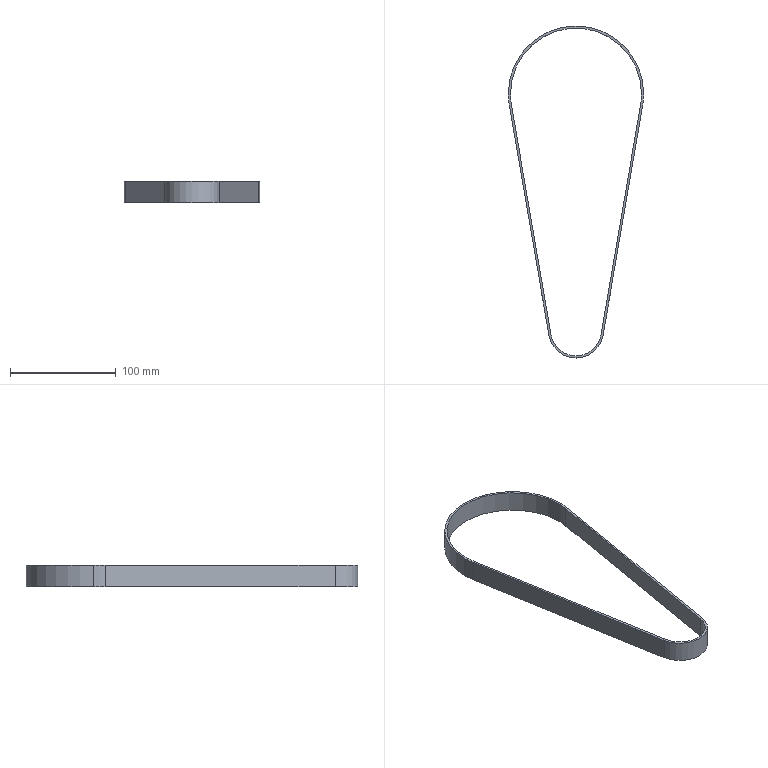Part | SolidWorks | features ExtruThin 1 | 1 solid | 14 faces | box 128 x 314 x 20 mm | volume 29237 mm3 | cylinder 8 | plane 6 | commonest cylinder face diameters 124 x3 128 x3 48 x1 52 x1
STEP:
#1=CARTESIAN_POINT('',(61.101,-10.518,20.));
#2=VERTEX_POINT('',#1);
#3=CARTESIAN_POINT('',(62.,0.,20.));
#4=VERTEX_POINT('',#3);
#5=CARTESIAN_POINT('',(0.,0.,20.));
#6=DIRECTION('',(0.,0.,1.));
#7=DIRECTION('',(1.,0.,0.));
#8=AXIS2_PLACEMENT_3D('',#5,#6,#7);
#9=CIRCLE('',#8,62.);
#10=EDGE_CURVE('',#2,#4,#9,.T.);
#11=ORIENTED_EDGE('',*,*,#10,.T.);
#12=CARTESIAN_POINT('',(62.,0.,0.));
#13=VERTEX_POINT('',#12);
#14=CARTESIAN_POINT('',(62.,0.,20.));
#15=DIRECTION('',(0.,0.,-1.));
#16=VECTOR('',#15,1000.);
#17=LINE('',#14,#16);
#18=EDGE_CURVE('',#4,#13,#17,.T.);
#19=ORIENTED_EDGE('',*,*,#18,.T.);
#20=CARTESIAN_POINT('',(61.101,-10.518,0.));
#21=VERTEX_POINT('',#20);
#22=CARTESIAN_POINT('',(0.,0.,0.));
#23=DIRECTION('',(0.,0.,1.));
#24=DIRECTION('',(1.,0.,0.));
#25=AXIS2_PLACEMENT_3D('',#22,#23,#24);
#26=CIRCLE('',#25,62.);
#27=EDGE_CURVE('',#21,#13,#26,.T.);
#28=ORIENTED_EDGE('',*,*,#27,.F.);
#29=CARTESIAN_POINT('',(61.101,-10.518,20.));
#30=DIRECTION('',(0.,0.,-1.));
#31=VECTOR('',#30,1000.);
#32=LINE('',#29,#31);
#33=EDGE_CURVE('',#2,#21,#32,.T.);
#34=ORIENTED_EDGE('',*,*,#33,.F.);
#35=EDGE_LOOP('',(#11,#19,#28,#34));
#36=FACE_OUTER_BOUND('',#35,.T.);
#37=CARTESIAN_POINT('',(0.,0.,20.));
#38=DIRECTION('',(0.,0.,-1.));
#39=DIRECTION('',(-1.,0.,0.));
#40=AXIS2_PLACEMENT_3D('',#37,#38,#39);
#41=CYLINDRICAL_SURFACE('',#40,62.);
#42=ADVANCED_FACE('',(#36),#41,.F.);
#43=ORIENTED_EDGE('',*,*,#18,.F.);
#44=CARTESIAN_POINT('',(-62.,0.,20.));
#45=VERTEX_POINT('',#44);
#46=CARTESIAN_POINT('',(0.,0.,20.));
#47=DIRECTION('',(0.,0.,1.));
#48=DIRECTION('',(1.,0.,0.));
#49=AXIS2_PLACEMENT_3D('',#46,#47,#48);
#50=CIRCLE('',#49,62.);
#51=EDGE_CURVE('',#4,#45,#50,.T.);
#52=ORIENTED_EDGE('',*,*,#51,.T.);
#53=CARTESIAN_POINT('',(-62.,0.,0.));
#54=VERTEX_POINT('',#53);
#55=CARTESIAN_POINT('',(-62.,0.,20.));
#56=DIRECTION('',(0.,0.,-1.));
#57=VECTOR('',#56,1000.);
#58=LINE('',#55,#57);
#59=EDGE_CURVE('',#45,#54,#58,.T.);
#60=ORIENTED_EDGE('',*,*,#59,.T.);
#61=CARTESIAN_POINT('',(0.,0.,0.));
#62=DIRECTION('',(0.,0.,1.));
#63=DIRECTION('',(1.,0.,0.));
#64=AXIS2_PLACEMENT_3D('',#61,#62,#63);
#65=CIRCLE('',#64,62.);
#66=EDGE_CURVE('',#13,#54,#65,.T.);
#67=ORIENTED_EDGE('',*,*,#66,.F.);
#68=EDGE_LOOP('',(#43,#52,#60,#67));
#69=FACE_OUTER_BOUND('',#68,.T.);
#70=CARTESIAN_POINT('',(0.,0.,20.));
#71=DIRECTION('',(0.,0.,-1.));
#72=DIRECTION('',(-1.,0.,0.));
#73=AXIS2_PLACEMENT_3D('',#70,#71,#72);
#74=CYLINDRICAL_SURFACE('',#73,62.);
#75=ADVANCED_FACE('',(#69),#74,.F.);
#76=CARTESIAN_POINT('',(64.,0.,20.));
#77=VERTEX_POINT('',#76);
#78=CARTESIAN_POINT('',(-64.,0.,20.));
#79=VERTEX_POINT('',#78);
#80=CARTESIAN_POINT('',(0.,0.,20.));
#81=DIRECTION('',(0.,0.,1.));
#82=DIRECTION('',(1.,0.,0.));
#83=AXIS2_PLACEMENT_3D('',#80,#81,#82);
#84=CIRCLE('',#83,64.);
#85=EDGE_CURVE('',#77,#79,#84,.T.);
#86=ORIENTED_EDGE('',*,*,#85,.F.);
#87=CARTESIAN_POINT('',(64.,0.,0.));
#88=VERTEX_POINT('',#87);
#89=CARTESIAN_POINT('',(64.,0.,20.));
#90=DIRECTION('',(0.,0.,-1.));
#91=VECTOR('',#90,1000.);
#92=LINE('',#89,#91);
#93=EDGE_CURVE('',#77,#88,#92,.T.);
#94=ORIENTED_EDGE('',*,*,#93,.T.);
#95=CARTESIAN_POINT('',(-64.,0.,0.));
#96=VERTEX_POINT('',#95);
#97=CARTESIAN_POINT('',(0.,0.,0.));
#98=DIRECTION('',(0.,0.,1.));
#99=DIRECTION('',(1.,0.,0.));
#100=AXIS2_PLACEMENT_3D('',#97,#98,#99);
#101=CIRCLE('',#100,64.);
#102=EDGE_CURVE('',#88,#96,#101,.T.);
#103=ORIENTED_EDGE('',*,*,#102,.T.);
#104=CARTESIAN_POINT('',(-64.,0.,20.));
#105=DIRECTION('',(0.,0.,-1.));
#106=VECTOR('',#105,1000.);
#107=LINE('',#104,#106);
#108=EDGE_CURVE('',#79,#96,#107,.T.);
#109=ORIENTED_EDGE('',*,*,#108,.F.);
#110=EDGE_LOOP('',(#86,#94,#103,#109));
#111=FACE_OUTER_BOUND('',#110,.T.);
#112=CARTESIAN_POINT('',(0.,0.,20.));
#113=DIRECTION('',(0.,0.,-1.));
#114=DIRECTION('',(-1.,0.,0.));
#115=AXIS2_PLACEMENT_3D('',#112,#113,#114);
#116=CYLINDRICAL_SURFACE('',#115,64.);
#117=ADVANCED_FACE('',(#111),#116,.T.);
#118=CARTESIAN_POINT('',(-63.072,-10.857,20.));
#119=VERTEX_POINT('',#118);
#120=CARTESIAN_POINT('',(0.,0.,20.));
#121=DIRECTION('',(0.,0.,1.));
#122=DIRECTION('',(1.,0.,0.));
#123=AXIS2_PLACEMENT_3D('',#120,#121,#122);
#124=CIRCLE('',#123,64.);
#125=EDGE_CURVE('',#79,#119,#124,.T.);
#126=ORIENTED_EDGE('',*,*,#125,.F.);
#127=ORIENTED_EDGE('',*,*,#108,.T.);
#128=CARTESIAN_POINT('',(-63.072,-10.857,0.));
#129=VERTEX_POINT('',#128);
#130=CARTESIAN_POINT('',(0.,0.,0.));
#131=DIRECTION('',(0.,0.,1.));
#132=DIRECTION('',(1.,0.,0.));
#133=AXIS2_PLACEMENT_3D('',#130,#131,#132);
#134=CIRCLE('',#133,64.);
#135=EDGE_CURVE('',#96,#129,#134,.T.);
#136=ORIENTED_EDGE('',*,*,#135,.T.);
#137=CARTESIAN_POINT('',(-63.072,-10.857,20.));
#138=DIRECTION('',(0.,0.,-1.));
#139=VECTOR('',#138,1000.);
#140=LINE('',#137,#139);
#141=EDGE_CURVE('',#119,#129,#140,.T.);
#142=ORIENTED_EDGE('',*,*,#141,.F.);
#143=EDGE_LOOP('',(#126,#127,#136,#142));
#144=FACE_OUTER_BOUND('',#143,.T.);
#145=CARTESIAN_POINT('',(0.,0.,20.));
#146=DIRECTION('',(0.,0.,-1.));
#147=DIRECTION('',(-1.,0.,0.));
#148=AXIS2_PLACEMENT_3D('',#145,#146,#147);
#149=CYLINDRICAL_SURFACE('',#148,64.);
#150=ADVANCED_FACE('',(#144),#149,.T.);
#151=CARTESIAN_POINT('',(63.072,-10.857,20.));
#152=VERTEX_POINT('',#151);
#153=CARTESIAN_POINT('',(0.,0.,20.));
#154=DIRECTION('',(0.,0.,1.));
#155=DIRECTION('',(1.,0.,0.));
#156=AXIS2_PLACEMENT_3D('',#153,#154,#155);
#157=CIRCLE('',#156,64.);
#158=EDGE_CURVE('',#152,#77,#157,.T.);
#159=ORIENTED_EDGE('',*,*,#158,.T.);
#160=ORIENTED_EDGE('',*,*,#85,.T.);
#161=ORIENTED_EDGE('',*,*,#125,.T.);
#162=CARTESIAN_POINT('',(-25.623,-228.411,20.));
#163=VERTEX_POINT('',#162);
#164=CARTESIAN_POINT('',(-63.072,-10.857,20.));
#165=DIRECTION('',(0.1696,-0.9855,0.));
#166=VECTOR('',#165,1000.);
#167=LINE('',#164,#166);
#168=EDGE_CURVE('',#119,#163,#167,.T.);
#169=ORIENTED_EDGE('',*,*,#168,.T.);
#170=CARTESIAN_POINT('',(25.623,-228.411,20.));
#171=VERTEX_POINT('',#170);
#172=CARTESIAN_POINT('',(0.,-224.,20.));
#173=DIRECTION('',(0.,0.,1.));
#174=DIRECTION('',(1.,0.,0.));
#175=AXIS2_PLACEMENT_3D('',#172,#173,#174);
#176=CIRCLE('',#175,26.);
#177=EDGE_CURVE('',#163,#171,#176,.T.);
#178=ORIENTED_EDGE('',*,*,#177,.T.);
#179=CARTESIAN_POINT('',(63.072,-10.857,20.));
#180=DIRECTION('',(0.1696,0.9855,0.));
#181=VECTOR('',#180,1000.);
#182=LINE('',#179,#181);
#183=EDGE_CURVE('',#171,#152,#182,.T.);
#184=ORIENTED_EDGE('',*,*,#183,.T.);
#185=EDGE_LOOP('',(#159,#160,#161,#169,#178,#184));
#186=FACE_OUTER_BOUND('',#185,.T.);
#187=CARTESIAN_POINT('',(-61.101,-10.518,20.));
#188=VERTEX_POINT('',#187);
#189=CARTESIAN_POINT('',(-23.652,-228.071,20.));
#190=VERTEX_POINT('',#189);
#191=CARTESIAN_POINT('',(-61.101,-10.518,20.));
#192=DIRECTION('',(0.1696,-0.9855,0.));
#193=VECTOR('',#192,1000.);
#194=LINE('',#191,#193);
#195=EDGE_CURVE('',#188,#190,#194,.T.);
#196=ORIENTED_EDGE('',*,*,#195,.F.);
#197=CARTESIAN_POINT('',(0.,0.,20.));
#198=DIRECTION('',(0.,0.,1.));
#199=DIRECTION('',(1.,0.,0.));
#200=AXIS2_PLACEMENT_3D('',#197,#198,#199);
#201=CIRCLE('',#200,62.);
#202=EDGE_CURVE('',#45,#188,#201,.T.);
#203=ORIENTED_EDGE('',*,*,#202,.F.);
#204=ORIENTED_EDGE('',*,*,#51,.F.);
#205=ORIENTED_EDGE('',*,*,#10,.F.);
#206=CARTESIAN_POINT('',(23.652,-228.071,20.));
#207=VERTEX_POINT('',#206);
#208=CARTESIAN_POINT('',(61.101,-10.518,20.));
#209=DIRECTION('',(0.1696,0.9855,0.));
#210=VECTOR('',#209,1000.);
#211=LINE('',#208,#210);
#212=EDGE_CURVE('',#207,#2,#211,.T.);
#213=ORIENTED_EDGE('',*,*,#212,.F.);
#214=CARTESIAN_POINT('',(0.,-224.,20.));
#215=DIRECTION('',(0.,0.,1.));
#216=DIRECTION('',(1.,0.,0.));
#217=AXIS2_PLACEMENT_3D('',#214,#215,#216);
#218=CIRCLE('',#217,24.);
#219=EDGE_CURVE('',#190,#207,#218,.T.);
#220=ORIENTED_EDGE('',*,*,#219,.F.);
#221=EDGE_LOOP('',(#196,#203,#204,#205,#213,#220));
#222=FACE_BOUND('',#221,.T.);
#223=CARTESIAN_POINT('',(0.,0.,20.));
#224=DIRECTION('',(0.,0.,1.));
#225=DIRECTION('',(1.,0.,0.));
#226=AXIS2_PLACEMENT_3D('',#223,#224,#225);
#227=PLANE('',#226);
#228=ADVANCED_FACE('',(#186,#222),#227,.T.);
#229=CARTESIAN_POINT('',(63.072,-10.857,0.));
#230=VERTEX_POINT('',#229);
#231=CARTESIAN_POINT('',(0.,0.,0.));
#232=DIRECTION('',(0.,0.,1.));
#233=DIRECTION('',(1.,0.,0.));
#234=AXIS2_PLACEMENT_3D('',#231,#232,#233);
#235=CIRCLE('',#234,64.);
#236=EDGE_CURVE('',#230,#88,#235,.T.);
#237=ORIENTED_EDGE('',*,*,#236,.F.);
#238=CARTESIAN_POINT('',(25.623,-228.411,0.));
#239=VERTEX_POINT('',#238);
#240=CARTESIAN_POINT('',(63.072,-10.857,0.));
#241=DIRECTION('',(0.1696,0.9855,0.));
#242=VECTOR('',#241,1000.);
#243=LINE('',#240,#242);
#244=EDGE_CURVE('',#239,#230,#243,.T.);
#245=ORIENTED_EDGE('',*,*,#244,.F.);
#246=CARTESIAN_POINT('',(-25.623,-228.411,0.));
#247=VERTEX_POINT('',#246);
#248=CARTESIAN_POINT('',(0.,-224.,0.));
#249=DIRECTION('',(0.,0.,1.));
#250=DIRECTION('',(1.,0.,0.));
#251=AXIS2_PLACEMENT_3D('',#248,#249,#250);
#252=CIRCLE('',#251,26.);
#253=EDGE_CURVE('',#247,#239,#252,.T.);
#254=ORIENTED_EDGE('',*,*,#253,.F.);
#255=CARTESIAN_POINT('',(-63.072,-10.857,0.));
#256=DIRECTION('',(0.1696,-0.9855,0.));
#257=VECTOR('',#256,1000.);
#258=LINE('',#255,#257);
#259=EDGE_CURVE('',#129,#247,#258,.T.);
#260=ORIENTED_EDGE('',*,*,#259,.F.);
#261=ORIENTED_EDGE('',*,*,#135,.F.);
#262=ORIENTED_EDGE('',*,*,#102,.F.);
#263=EDGE_LOOP('',(#237,#245,#254,#260,#261,#262));
#264=FACE_OUTER_BOUND('',#263,.T.);
#265=ORIENTED_EDGE('',*,*,#27,.T.);
#266=ORIENTED_EDGE('',*,*,#66,.T.);
#267=CARTESIAN_POINT('',(-61.101,-10.518,0.));
#268=VERTEX_POINT('',#267);
#269=CARTESIAN_POINT('',(0.,0.,0.));
#270=DIRECTION('',(0.,0.,1.));
#271=DIRECTION('',(1.,0.,0.));
#272=AXIS2_PLACEMENT_3D('',#269,#270,#271);
#273=CIRCLE('',#272,62.);
#274=EDGE_CURVE('',#54,#268,#273,.T.);
#275=ORIENTED_EDGE('',*,*,#274,.T.);
#276=CARTESIAN_POINT('',(-23.652,-228.071,0.));
#277=VERTEX_POINT('',#276);
#278=CARTESIAN_POINT('',(-61.101,-10.518,0.));
#279=DIRECTION('',(0.1696,-0.9855,0.));
#280=VECTOR('',#279,1000.);
#281=LINE('',#278,#280);
#282=EDGE_CURVE('',#268,#277,#281,.T.);
#283=ORIENTED_EDGE('',*,*,#282,.T.);
#284=CARTESIAN_POINT('',(23.652,-228.071,0.));
#285=VERTEX_POINT('',#284);
#286=CARTESIAN_POINT('',(0.,-224.,0.));
#287=DIRECTION('',(0.,0.,1.));
#288=DIRECTION('',(1.,0.,0.));
#289=AXIS2_PLACEMENT_3D('',#286,#287,#288);
#290=CIRCLE('',#289,24.);
#291=EDGE_CURVE('',#277,#285,#290,.T.);
#292=ORIENTED_EDGE('',*,*,#291,.T.);
#293=CARTESIAN_POINT('',(61.101,-10.518,0.));
#294=DIRECTION('',(0.1696,0.9855,0.));
#295=VECTOR('',#294,1000.);
#296=LINE('',#293,#295);
#297=EDGE_CURVE('',#285,#21,#296,.T.);
#298=ORIENTED_EDGE('',*,*,#297,.T.);
#299=EDGE_LOOP('',(#265,#266,#275,#283,#292,#298));
#300=FACE_BOUND('',#299,.T.);
#301=CARTESIAN_POINT('',(0.,0.,0.));
#302=DIRECTION('',(0.,0.,1.));
#303=DIRECTION('',(1.,0.,0.));
#304=AXIS2_PLACEMENT_3D('',#301,#302,#303);
#305=PLANE('',#304);
#306=ADVANCED_FACE('',(#264,#300),#305,.F.);
#307=ORIENTED_EDGE('',*,*,#93,.F.);
#308=ORIENTED_EDGE('',*,*,#158,.F.);
#309=CARTESIAN_POINT('',(63.072,-10.857,20.));
#310=DIRECTION('',(0.,0.,-1.));
#311=VECTOR('',#310,1000.);
#312=LINE('',#309,#311);
#313=EDGE_CURVE('',#152,#230,#312,.T.);
#314=ORIENTED_EDGE('',*,*,#313,.T.);
#315=ORIENTED_EDGE('',*,*,#236,.T.);
#316=EDGE_LOOP('',(#307,#308,#314,#315));
#317=FACE_OUTER_BOUND('',#316,.T.);
#318=CARTESIAN_POINT('',(0.,0.,20.));
#319=DIRECTION('',(0.,0.,-1.));
#320=DIRECTION('',(-1.,0.,0.));
#321=AXIS2_PLACEMENT_3D('',#318,#319,#320);
#322=CYLINDRICAL_SURFACE('',#321,64.);
#323=ADVANCED_FACE('',(#317),#322,.T.);
#324=ORIENTED_EDGE('',*,*,#259,.T.);
#325=CARTESIAN_POINT('',(-25.623,-228.411,20.));
#326=DIRECTION('',(0.,0.,-1.));
#327=VECTOR('',#326,1000.);
#328=LINE('',#325,#327);
#329=EDGE_CURVE('',#163,#247,#328,.T.);
#330=ORIENTED_EDGE('',*,*,#329,.F.);
#331=ORIENTED_EDGE('',*,*,#168,.F.);
#332=ORIENTED_EDGE('',*,*,#141,.T.);
#333=EDGE_LOOP('',(#324,#330,#331,#332));
#334=FACE_OUTER_BOUND('',#333,.T.);
#335=CARTESIAN_POINT('',(-63.072,-10.857,20.));
#336=DIRECTION('',(0.9855,0.1696,0.));
#337=DIRECTION('',(-0.1696,0.9855,0.));
#338=AXIS2_PLACEMENT_3D('',#335,#336,#337);
#339=PLANE('',#338);
#340=ADVANCED_FACE('',(#334),#339,.F.);
#341=ORIENTED_EDGE('',*,*,#253,.T.);
#342=CARTESIAN_POINT('',(25.623,-228.411,20.));
#343=DIRECTION('',(0.,0.,-1.));
#344=VECTOR('',#343,1000.);
#345=LINE('',#342,#344);
#346=EDGE_CURVE('',#171,#239,#345,.T.);
#347=ORIENTED_EDGE('',*,*,#346,.F.);
#348=ORIENTED_EDGE('',*,*,#177,.F.);
#349=ORIENTED_EDGE('',*,*,#329,.T.);
#350=EDGE_LOOP('',(#341,#347,#348,#349));
#351=FACE_OUTER_BOUND('',#350,.T.);
#352=CARTESIAN_POINT('',(0.,-224.,20.));
#353=DIRECTION('',(0.,0.,-1.));
#354=DIRECTION('',(-1.,0.,0.));
#355=AXIS2_PLACEMENT_3D('',#352,#353,#354);
#356=CYLINDRICAL_SURFACE('',#355,26.);
#357=ADVANCED_FACE('',(#351),#356,.T.);
#358=ORIENTED_EDGE('',*,*,#244,.T.);
#359=ORIENTED_EDGE('',*,*,#313,.F.);
#360=ORIENTED_EDGE('',*,*,#183,.F.);
#361=ORIENTED_EDGE('',*,*,#346,.T.);
#362=EDGE_LOOP('',(#358,#359,#360,#361));
#363=FACE_OUTER_BOUND('',#362,.T.);
#364=CARTESIAN_POINT('',(63.072,-10.857,20.));
#365=DIRECTION('',(-0.9855,0.1696,0.));
#366=DIRECTION('',(-0.1696,-0.9855,0.));
#367=AXIS2_PLACEMENT_3D('',#364,#365,#366);
#368=PLANE('',#367);
#369=ADVANCED_FACE('',(#363),#368,.F.);
#370=ORIENTED_EDGE('',*,*,#59,.F.);
#371=ORIENTED_EDGE('',*,*,#202,.T.);
#372=CARTESIAN_POINT('',(-61.101,-10.518,20.));
#373=DIRECTION('',(0.,0.,-1.));
#374=VECTOR('',#373,1000.);
#375=LINE('',#372,#374);
#376=EDGE_CURVE('',#188,#268,#375,.T.);
#377=ORIENTED_EDGE('',*,*,#376,.T.);
#378=ORIENTED_EDGE('',*,*,#274,.F.);
#379=EDGE_LOOP('',(#370,#371,#377,#378));
#380=FACE_OUTER_BOUND('',#379,.T.);
#381=CARTESIAN_POINT('',(0.,0.,20.));
#382=DIRECTION('',(0.,0.,-1.));
#383=DIRECTION('',(-1.,0.,0.));
#384=AXIS2_PLACEMENT_3D('',#381,#382,#383);
#385=CYLINDRICAL_SURFACE('',#384,62.);
#386=ADVANCED_FACE('',(#380),#385,.F.);
#387=ORIENTED_EDGE('',*,*,#282,.F.);
#388=ORIENTED_EDGE('',*,*,#376,.F.);
#389=ORIENTED_EDGE('',*,*,#195,.T.);
#390=CARTESIAN_POINT('',(-23.652,-228.071,20.));
#391=DIRECTION('',(0.,0.,-1.));
#392=VECTOR('',#391,1000.);
#393=LINE('',#390,#392);
#394=EDGE_CURVE('',#190,#277,#393,.T.);
#395=ORIENTED_EDGE('',*,*,#394,.T.);
#396=EDGE_LOOP('',(#387,#388,#389,#395));
#397=FACE_OUTER_BOUND('',#396,.T.);
#398=CARTESIAN_POINT('',(-61.101,-10.518,20.));
#399=DIRECTION('',(0.9855,0.1696,0.));
#400=DIRECTION('',(-0.1696,0.9855,0.));
#401=AXIS2_PLACEMENT_3D('',#398,#399,#400);
#402=PLANE('',#401);
#403=ADVANCED_FACE('',(#397),#402,.T.);
#404=ORIENTED_EDGE('',*,*,#291,.F.);
#405=ORIENTED_EDGE('',*,*,#394,.F.);
#406=ORIENTED_EDGE('',*,*,#219,.T.);
#407=CARTESIAN_POINT('',(23.652,-228.071,20.));
#408=DIRECTION('',(0.,0.,-1.));
#409=VECTOR('',#408,1000.);
#410=LINE('',#407,#409);
#411=EDGE_CURVE('',#207,#285,#410,.T.);
#412=ORIENTED_EDGE('',*,*,#411,.T.);
#413=EDGE_LOOP('',(#404,#405,#406,#412));
#414=FACE_OUTER_BOUND('',#413,.T.);
#415=CARTESIAN_POINT('',(0.,-224.,20.));
#416=DIRECTION('',(0.,0.,-1.));
#417=DIRECTION('',(-1.,0.,0.));
#418=AXIS2_PLACEMENT_3D('',#415,#416,#417);
#419=CYLINDRICAL_SURFACE('',#418,24.);
#420=ADVANCED_FACE('',(#414),#419,.F.);
#421=ORIENTED_EDGE('',*,*,#297,.F.);
#422=ORIENTED_EDGE('',*,*,#411,.F.);
#423=ORIENTED_EDGE('',*,*,#212,.T.);
#424=ORIENTED_EDGE('',*,*,#33,.T.);
#425=EDGE_LOOP('',(#421,#422,#423,#424));
#426=FACE_OUTER_BOUND('',#425,.T.);
#427=CARTESIAN_POINT('',(61.101,-10.518,20.));
#428=DIRECTION('',(-0.9855,0.1696,0.));
#429=DIRECTION('',(-0.1696,-0.9855,0.));
#430=AXIS2_PLACEMENT_3D('',#427,#428,#429);
#431=PLANE('',#430);
#432=ADVANCED_FACE('',(#426),#431,.T.);
#433=CLOSED_SHELL('',(#42,#75,#117,#150,#228,#306,#323,#340,#357,#369,#386,#403,#420,#432));
#434=MANIFOLD_SOLID_BREP('',#433);
#435=CARTESIAN_POINT('',(0.,0.,0.));
#436=DIRECTION('',(0.,0.,1.));
#437=DIRECTION('',(1.,0.,0.));
#438=AXIS2_PLACEMENT_3D('',#435,#436,#437);
#439=(LENGTH_UNIT()NAMED_UNIT(*)SI_UNIT(.MILLI.,.METRE.));
#440=UNCERTAINTY_MEASURE_WITH_UNIT(LENGTH_MEASURE(0.00001),#439,'','');
#441=(NAMED_UNIT(*)PLANE_ANGLE_UNIT()SI_UNIT($,.RADIAN.));
#442=(NAMED_UNIT(*)SI_UNIT($,.STERADIAN.)SOLID_ANGLE_UNIT());
#443=(GEOMETRIC_REPRESENTATION_CONTEXT(3)GLOBAL_UNCERTAINTY_ASSIGNED_CONTEXT((#440))GLOBAL_UNIT_ASSIGNED_CONTEXT((#439,#441,#442))REPRESENTATION_CONTEXT('',''));
#444=ADVANCED_BREP_SHAPE_REPRESENTATION('',(#434,#438),#443);